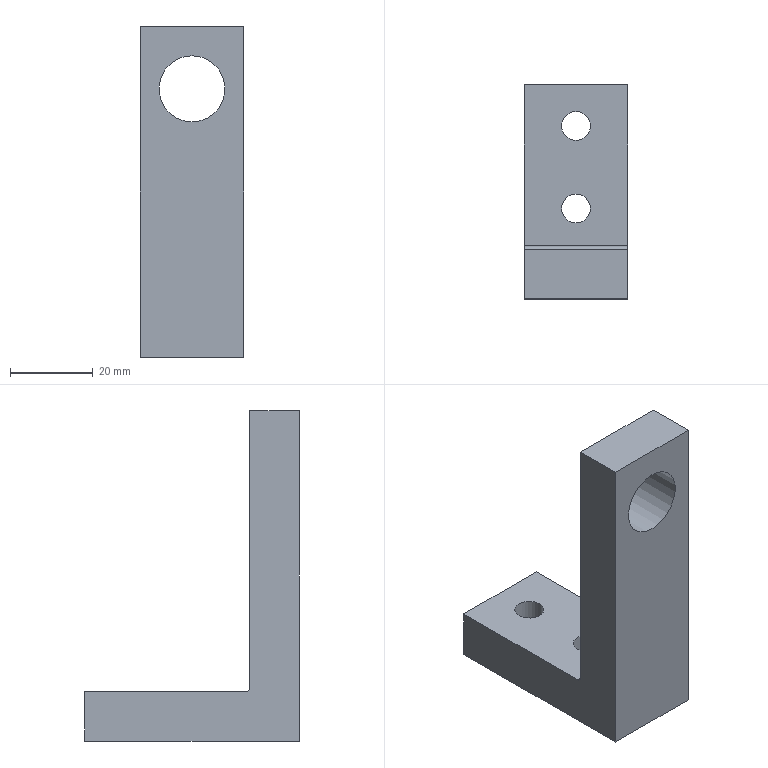Part | NX | features 5003_218_Panel feed stopper 2 | 1 solid | 12 faces | box 25 x 52 x 80 mm | volume 32669 mm3 | plane 8 | cylinder 4 | commonest cylinder face diameters 7 x2 2 x1 16 x1
STEP:
#1=CARTESIAN_POINT('',(-152.975,25.9,-107.));
#2=VERTEX_POINT('',#1);
#3=CARTESIAN_POINT('',(-152.975,13.9,-107.));
#4=VERTEX_POINT('',#3);
#5=CARTESIAN_POINT('',(-152.975,25.9,-107.));
#6=DIRECTION('',(0.,-1.,0.));
#7=VECTOR('',#6,1000.);
#8=LINE('',#5,#7);
#9=EDGE_CURVE('',#2,#4,#8,.T.);
#10=ORIENTED_EDGE('',*,*,#9,.T.);
#11=CARTESIAN_POINT('',(-127.975,13.9,-107.));
#12=VERTEX_POINT('',#11);
#13=CARTESIAN_POINT('',(-127.975,13.9,-107.));
#14=DIRECTION('',(-1.,0.,0.));
#15=VECTOR('',#14,1000.);
#16=LINE('',#13,#15);
#17=EDGE_CURVE('',#12,#4,#16,.T.);
#18=ORIENTED_EDGE('',*,*,#17,.F.);
#19=CARTESIAN_POINT('',(-127.975,25.9,-107.));
#20=VERTEX_POINT('',#19);
#21=CARTESIAN_POINT('',(-127.975,25.9,-107.));
#22=DIRECTION('',(0.,-1.,0.));
#23=VECTOR('',#22,1000.);
#24=LINE('',#21,#23);
#25=EDGE_CURVE('',#20,#12,#24,.T.);
#26=ORIENTED_EDGE('',*,*,#25,.F.);
#27=CARTESIAN_POINT('',(-127.975,25.9,-107.));
#28=DIRECTION('',(-1.,0.,0.));
#29=VECTOR('',#28,1000.);
#30=LINE('',#27,#29);
#31=EDGE_CURVE('',#20,#2,#30,.T.);
#32=ORIENTED_EDGE('',*,*,#31,.T.);
#33=EDGE_LOOP('',(#10,#18,#26,#32));
#34=FACE_BOUND('',#33,.T.);
#35=CARTESIAN_POINT('',(-127.975,25.9,-107.));
#36=DIRECTION('',(0.,0.,-1.));
#37=DIRECTION('',(0.,1.,0.));
#38=AXIS2_PLACEMENT_3D('',#35,#36,#37);
#39=PLANE('',#38);
#40=ADVANCED_FACE('',(#34),#39,.F.);
#41=CARTESIAN_POINT('',(-140.475,13.9,-114.));
#42=VERTEX_POINT('',#41);
#43=CARTESIAN_POINT('',(-140.475,13.9,-122.));
#44=DIRECTION('',(0.,1.,0.));
#45=DIRECTION('',(0.,0.,1.));
#46=AXIS2_PLACEMENT_3D('',#43,#44,#45);
#47=CIRCLE('',#46,8.);
#48=EDGE_CURVE('',#42,#42,#47,.T.);
#49=ORIENTED_EDGE('',*,*,#48,.T.);
#50=EDGE_LOOP('',(#49));
#51=FACE_BOUND('',#50,.T.);
#52=CARTESIAN_POINT('',(-152.975,13.9,-187.));
#53=VERTEX_POINT('',#52);
#54=CARTESIAN_POINT('',(-152.975,13.9,-107.));
#55=DIRECTION('',(0.,0.,-1.));
#56=VECTOR('',#55,1000.);
#57=LINE('',#54,#56);
#58=EDGE_CURVE('',#4,#53,#57,.T.);
#59=ORIENTED_EDGE('',*,*,#58,.T.);
#60=CARTESIAN_POINT('',(-127.975,13.9,-187.));
#61=VERTEX_POINT('',#60);
#62=CARTESIAN_POINT('',(-127.975,13.9,-187.));
#63=DIRECTION('',(-1.,0.,0.));
#64=VECTOR('',#63,1000.);
#65=LINE('',#62,#64);
#66=EDGE_CURVE('',#61,#53,#65,.T.);
#67=ORIENTED_EDGE('',*,*,#66,.F.);
#68=CARTESIAN_POINT('',(-127.975,13.9,-107.));
#69=DIRECTION('',(0.,0.,-1.));
#70=VECTOR('',#69,1000.);
#71=LINE('',#68,#70);
#72=EDGE_CURVE('',#12,#61,#71,.T.);
#73=ORIENTED_EDGE('',*,*,#72,.F.);
#74=ORIENTED_EDGE('',*,*,#17,.T.);
#75=EDGE_LOOP('',(#59,#67,#73,#74));
#76=FACE_BOUND('',#75,.T.);
#77=CARTESIAN_POINT('',(-127.975,13.9,-107.));
#78=DIRECTION('',(0.,1.,0.));
#79=DIRECTION('',(0.,0.,1.));
#80=AXIS2_PLACEMENT_3D('',#77,#78,#79);
#81=PLANE('',#80);
#82=ADVANCED_FACE('',(#51,#76),#81,.F.);
#83=CARTESIAN_POINT('',(-140.475,52.4,-187.));
#84=VERTEX_POINT('',#83);
#85=CARTESIAN_POINT('',(-140.475,55.9,-187.));
#86=DIRECTION('',(0.,0.,1.));
#87=DIRECTION('',(0.,-1.,0.));
#88=AXIS2_PLACEMENT_3D('',#85,#86,#87);
#89=CIRCLE('',#88,3.5);
#90=EDGE_CURVE('',#84,#84,#89,.T.);
#91=ORIENTED_EDGE('',*,*,#90,.T.);
#92=EDGE_LOOP('',(#91));
#93=FACE_BOUND('',#92,.T.);
#94=CARTESIAN_POINT('',(-140.475,32.4,-187.));
#95=VERTEX_POINT('',#94);
#96=CARTESIAN_POINT('',(-140.475,35.9,-187.));
#97=DIRECTION('',(0.,0.,1.));
#98=DIRECTION('',(0.,-1.,0.));
#99=AXIS2_PLACEMENT_3D('',#96,#97,#98);
#100=CIRCLE('',#99,3.5);
#101=EDGE_CURVE('',#95,#95,#100,.T.);
#102=ORIENTED_EDGE('',*,*,#101,.T.);
#103=EDGE_LOOP('',(#102));
#104=FACE_BOUND('',#103,.T.);
#105=CARTESIAN_POINT('',(-152.975,65.9,-187.));
#106=VERTEX_POINT('',#105);
#107=CARTESIAN_POINT('',(-152.975,13.9,-187.));
#108=DIRECTION('',(0.,1.,0.));
#109=VECTOR('',#108,1000.);
#110=LINE('',#107,#109);
#111=EDGE_CURVE('',#53,#106,#110,.T.);
#112=ORIENTED_EDGE('',*,*,#111,.T.);
#113=CARTESIAN_POINT('',(-127.975,65.9,-187.));
#114=VERTEX_POINT('',#113);
#115=CARTESIAN_POINT('',(-127.975,65.9,-187.));
#116=DIRECTION('',(-1.,0.,0.));
#117=VECTOR('',#116,1000.);
#118=LINE('',#115,#117);
#119=EDGE_CURVE('',#114,#106,#118,.T.);
#120=ORIENTED_EDGE('',*,*,#119,.F.);
#121=CARTESIAN_POINT('',(-127.975,13.9,-187.));
#122=DIRECTION('',(0.,1.,0.));
#123=VECTOR('',#122,1000.);
#124=LINE('',#121,#123);
#125=EDGE_CURVE('',#61,#114,#124,.T.);
#126=ORIENTED_EDGE('',*,*,#125,.F.);
#127=ORIENTED_EDGE('',*,*,#66,.T.);
#128=EDGE_LOOP('',(#112,#120,#126,#127));
#129=FACE_BOUND('',#128,.T.);
#130=CARTESIAN_POINT('',(-127.975,13.9,-187.));
#131=DIRECTION('',(0.,0.,1.));
#132=DIRECTION('',(0.,-1.,0.));
#133=AXIS2_PLACEMENT_3D('',#130,#131,#132);
#134=PLANE('',#133);
#135=ADVANCED_FACE('',(#93,#104,#129),#134,.F.);
#136=CARTESIAN_POINT('',(-152.975,65.9,-175.));
#137=VERTEX_POINT('',#136);
#138=CARTESIAN_POINT('',(-152.975,65.9,-187.));
#139=DIRECTION('',(0.,0.,1.));
#140=VECTOR('',#139,1000.);
#141=LINE('',#138,#140);
#142=EDGE_CURVE('',#106,#137,#141,.T.);
#143=ORIENTED_EDGE('',*,*,#142,.T.);
#144=CARTESIAN_POINT('',(-127.975,65.9,-175.));
#145=VERTEX_POINT('',#144);
#146=CARTESIAN_POINT('',(-127.975,65.9,-175.));
#147=DIRECTION('',(-1.,0.,0.));
#148=VECTOR('',#147,1000.);
#149=LINE('',#146,#148);
#150=EDGE_CURVE('',#145,#137,#149,.T.);
#151=ORIENTED_EDGE('',*,*,#150,.F.);
#152=CARTESIAN_POINT('',(-127.975,65.9,-187.));
#153=DIRECTION('',(0.,0.,1.));
#154=VECTOR('',#153,1000.);
#155=LINE('',#152,#154);
#156=EDGE_CURVE('',#114,#145,#155,.T.);
#157=ORIENTED_EDGE('',*,*,#156,.F.);
#158=ORIENTED_EDGE('',*,*,#119,.T.);
#159=EDGE_LOOP('',(#143,#151,#157,#158));
#160=FACE_BOUND('',#159,.T.);
#161=CARTESIAN_POINT('',(-127.975,65.9,-187.));
#162=DIRECTION('',(0.,-1.,0.));
#163=DIRECTION('',(1.,0.,0.));
#164=AXIS2_PLACEMENT_3D('',#161,#162,#163);
#165=PLANE('',#164);
#166=ADVANCED_FACE('',(#160),#165,.F.);
#167=CARTESIAN_POINT('',(-140.475,52.4,-175.));
#168=VERTEX_POINT('',#167);
#169=CARTESIAN_POINT('',(-140.475,55.9,-175.));
#170=DIRECTION('',(0.,0.,1.));
#171=DIRECTION('',(0.,-1.,0.));
#172=AXIS2_PLACEMENT_3D('',#169,#170,#171);
#173=CIRCLE('',#172,3.5);
#174=EDGE_CURVE('',#168,#168,#173,.T.);
#175=ORIENTED_EDGE('',*,*,#174,.F.);
#176=EDGE_LOOP('',(#175));
#177=FACE_BOUND('',#176,.T.);
#178=CARTESIAN_POINT('',(-140.475,32.4,-175.));
#179=VERTEX_POINT('',#178);
#180=CARTESIAN_POINT('',(-140.475,35.9,-175.));
#181=DIRECTION('',(0.,0.,1.));
#182=DIRECTION('',(0.,-1.,0.));
#183=AXIS2_PLACEMENT_3D('',#180,#181,#182);
#184=CIRCLE('',#183,3.5);
#185=EDGE_CURVE('',#179,#179,#184,.T.);
#186=ORIENTED_EDGE('',*,*,#185,.F.);
#187=EDGE_LOOP('',(#186));
#188=FACE_BOUND('',#187,.T.);
#189=CARTESIAN_POINT('',(-152.975,26.9,-175.));
#190=VERTEX_POINT('',#189);
#191=CARTESIAN_POINT('',(-152.975,65.9,-175.));
#192=DIRECTION('',(0.,-1.,0.));
#193=VECTOR('',#192,1000.);
#194=LINE('',#191,#193);
#195=EDGE_CURVE('',#137,#190,#194,.T.);
#196=ORIENTED_EDGE('',*,*,#195,.T.);
#197=CARTESIAN_POINT('',(-127.975,26.9,-175.));
#198=VERTEX_POINT('',#197);
#199=CARTESIAN_POINT('',(-127.975,26.9,-175.));
#200=DIRECTION('',(-1.,0.,0.));
#201=VECTOR('',#200,1000.);
#202=LINE('',#199,#201);
#203=EDGE_CURVE('',#190,#198,#202,.F.);
#204=ORIENTED_EDGE('',*,*,#203,.T.);
#205=CARTESIAN_POINT('',(-127.975,65.9,-175.));
#206=DIRECTION('',(0.,-1.,0.));
#207=VECTOR('',#206,1000.);
#208=LINE('',#205,#207);
#209=EDGE_CURVE('',#145,#198,#208,.T.);
#210=ORIENTED_EDGE('',*,*,#209,.F.);
#211=ORIENTED_EDGE('',*,*,#150,.T.);
#212=EDGE_LOOP('',(#196,#204,#210,#211));
#213=FACE_BOUND('',#212,.T.);
#214=CARTESIAN_POINT('',(-127.975,65.9,-175.));
#215=DIRECTION('',(0.,0.,-1.));
#216=DIRECTION('',(0.,1.,0.));
#217=AXIS2_PLACEMENT_3D('',#214,#215,#216);
#218=PLANE('',#217);
#219=ADVANCED_FACE('',(#177,#188,#213),#218,.F.);
#220=CARTESIAN_POINT('',(-140.475,25.9,-114.));
#221=VERTEX_POINT('',#220);
#222=CARTESIAN_POINT('',(-140.475,25.9,-122.));
#223=DIRECTION('',(0.,1.,0.));
#224=DIRECTION('',(0.,0.,1.));
#225=AXIS2_PLACEMENT_3D('',#222,#223,#224);
#226=CIRCLE('',#225,8.);
#227=EDGE_CURVE('',#221,#221,#226,.T.);
#228=ORIENTED_EDGE('',*,*,#227,.F.);
#229=EDGE_LOOP('',(#228));
#230=FACE_BOUND('',#229,.T.);
#231=CARTESIAN_POINT('',(-127.975,25.9,-174.));
#232=VERTEX_POINT('',#231);
#233=CARTESIAN_POINT('',(-127.975,25.9,-175.));
#234=DIRECTION('',(0.,0.,1.));
#235=VECTOR('',#234,1000.);
#236=LINE('',#233,#235);
#237=EDGE_CURVE('',#232,#20,#236,.T.);
#238=ORIENTED_EDGE('',*,*,#237,.F.);
#239=CARTESIAN_POINT('',(-152.975,25.9,-174.));
#240=VERTEX_POINT('',#239);
#241=CARTESIAN_POINT('',(-152.975,25.9,-174.));
#242=DIRECTION('',(-1.,0.,0.));
#243=VECTOR('',#242,1000.);
#244=LINE('',#241,#243);
#245=EDGE_CURVE('',#232,#240,#244,.T.);
#246=ORIENTED_EDGE('',*,*,#245,.T.);
#247=CARTESIAN_POINT('',(-152.975,25.9,-175.));
#248=DIRECTION('',(0.,0.,1.));
#249=VECTOR('',#248,1000.);
#250=LINE('',#247,#249);
#251=EDGE_CURVE('',#240,#2,#250,.T.);
#252=ORIENTED_EDGE('',*,*,#251,.T.);
#253=ORIENTED_EDGE('',*,*,#31,.F.);
#254=EDGE_LOOP('',(#238,#246,#252,#253));
#255=FACE_BOUND('',#254,.T.);
#256=CARTESIAN_POINT('',(-127.975,25.9,-175.));
#257=DIRECTION('',(0.,-1.,0.));
#258=DIRECTION('',(0.,0.,-1.));
#259=AXIS2_PLACEMENT_3D('',#256,#257,#258);
#260=PLANE('',#259);
#261=ADVANCED_FACE('',(#230,#255),#260,.F.);
#262=ORIENTED_EDGE('',*,*,#25,.T.);
#263=ORIENTED_EDGE('',*,*,#72,.T.);
#264=ORIENTED_EDGE('',*,*,#125,.T.);
#265=ORIENTED_EDGE('',*,*,#156,.T.);
#266=ORIENTED_EDGE('',*,*,#209,.T.);
#267=CARTESIAN_POINT('',(-127.975,26.9,-174.));
#268=DIRECTION('',(1.,0.,0.));
#269=DIRECTION('',(0.,1.,0.));
#270=AXIS2_PLACEMENT_3D('',#267,#268,#269);
#271=CIRCLE('',#270,1.);
#272=EDGE_CURVE('',#198,#232,#271,.F.);
#273=ORIENTED_EDGE('',*,*,#272,.T.);
#274=ORIENTED_EDGE('',*,*,#237,.T.);
#275=EDGE_LOOP('',(#262,#263,#264,#265,#266,#273,#274));
#276=FACE_BOUND('',#275,.T.);
#277=CARTESIAN_POINT('',(-127.975,13.9,-187.));
#278=DIRECTION('',(1.,0.,0.));
#279=DIRECTION('',(0.,1.,0.));
#280=AXIS2_PLACEMENT_3D('',#277,#278,#279);
#281=PLANE('',#280);
#282=ADVANCED_FACE('',(#276),#281,.T.);
#283=ORIENTED_EDGE('',*,*,#9,.F.);
#284=ORIENTED_EDGE('',*,*,#251,.F.);
#285=CARTESIAN_POINT('',(-152.975,26.9,-174.));
#286=DIRECTION('',(1.,0.,0.));
#287=DIRECTION('',(0.,1.,0.));
#288=AXIS2_PLACEMENT_3D('',#285,#286,#287);
#289=CIRCLE('',#288,1.);
#290=EDGE_CURVE('',#240,#190,#289,.T.);
#291=ORIENTED_EDGE('',*,*,#290,.T.);
#292=ORIENTED_EDGE('',*,*,#195,.F.);
#293=ORIENTED_EDGE('',*,*,#142,.F.);
#294=ORIENTED_EDGE('',*,*,#111,.F.);
#295=ORIENTED_EDGE('',*,*,#58,.F.);
#296=EDGE_LOOP('',(#283,#284,#291,#292,#293,#294,#295));
#297=FACE_BOUND('',#296,.T.);
#298=CARTESIAN_POINT('',(-152.975,13.9,-187.));
#299=DIRECTION('',(1.,0.,0.));
#300=DIRECTION('',(0.,1.,0.));
#301=AXIS2_PLACEMENT_3D('',#298,#299,#300);
#302=PLANE('',#301);
#303=ADVANCED_FACE('',(#297),#302,.F.);
#304=ORIENTED_EDGE('',*,*,#48,.F.);
#305=EDGE_LOOP('',(#304));
#306=FACE_BOUND('',#305,.T.);
#307=ORIENTED_EDGE('',*,*,#227,.T.);
#308=EDGE_LOOP('',(#307));
#309=FACE_BOUND('',#308,.T.);
#310=CARTESIAN_POINT('',(-140.475,25.9,-122.));
#311=DIRECTION('',(0.,1.,0.));
#312=DIRECTION('',(0.,0.,1.));
#313=AXIS2_PLACEMENT_3D('',#310,#311,#312);
#314=CYLINDRICAL_SURFACE('',#313,8.);
#315=ADVANCED_FACE('',(#306,#309),#314,.F.);
#316=ORIENTED_EDGE('',*,*,#101,.F.);
#317=EDGE_LOOP('',(#316));
#318=FACE_BOUND('',#317,.T.);
#319=ORIENTED_EDGE('',*,*,#185,.T.);
#320=EDGE_LOOP('',(#319));
#321=FACE_BOUND('',#320,.T.);
#322=CARTESIAN_POINT('',(-140.475,35.9,-175.));
#323=DIRECTION('',(0.,0.,1.));
#324=DIRECTION('',(0.,-1.,0.));
#325=AXIS2_PLACEMENT_3D('',#322,#323,#324);
#326=CYLINDRICAL_SURFACE('',#325,3.5);
#327=ADVANCED_FACE('',(#318,#321),#326,.F.);
#328=ORIENTED_EDGE('',*,*,#90,.F.);
#329=EDGE_LOOP('',(#328));
#330=FACE_BOUND('',#329,.T.);
#331=ORIENTED_EDGE('',*,*,#174,.T.);
#332=EDGE_LOOP('',(#331));
#333=FACE_BOUND('',#332,.T.);
#334=CARTESIAN_POINT('',(-140.475,55.9,-175.));
#335=DIRECTION('',(0.,0.,1.));
#336=DIRECTION('',(0.,-1.,0.));
#337=AXIS2_PLACEMENT_3D('',#334,#335,#336);
#338=CYLINDRICAL_SURFACE('',#337,3.5);
#339=ADVANCED_FACE('',(#330,#333),#338,.F.);
#340=ORIENTED_EDGE('',*,*,#272,.F.);
#341=ORIENTED_EDGE('',*,*,#203,.F.);
#342=ORIENTED_EDGE('',*,*,#290,.F.);
#343=ORIENTED_EDGE('',*,*,#245,.F.);
#344=EDGE_LOOP('',(#340,#341,#342,#343));
#345=FACE_BOUND('',#344,.T.);
#346=CARTESIAN_POINT('',(-127.975,26.9,-174.));
#347=DIRECTION('',(1.,0.,0.));
#348=DIRECTION('',(0.,1.,0.));
#349=AXIS2_PLACEMENT_3D('',#346,#347,#348);
#350=CYLINDRICAL_SURFACE('',#349,1.);
#351=ADVANCED_FACE('',(#345),#350,.F.);
#352=CLOSED_SHELL('',(#40,#82,#135,#166,#219,#261,#282,#303,#315,#327,#339,#351));
#353=MANIFOLD_SOLID_BREP('',#352);
#354=(LENGTH_UNIT()NAMED_UNIT(*)SI_UNIT(.MILLI.,.METRE.));
#355=UNCERTAINTY_MEASURE_WITH_UNIT(LENGTH_MEASURE(0.00001),#354,'','');
#356=(NAMED_UNIT(*)PLANE_ANGLE_UNIT()SI_UNIT($,.RADIAN.));
#357=(NAMED_UNIT(*)SI_UNIT($,.STERADIAN.)SOLID_ANGLE_UNIT());
#358=(GEOMETRIC_REPRESENTATION_CONTEXT(3)GLOBAL_UNCERTAINTY_ASSIGNED_CONTEXT((#355))GLOBAL_UNIT_ASSIGNED_CONTEXT((#354,#356,#357))REPRESENTATION_CONTEXT('',''));
#359=ADVANCED_BREP_SHAPE_REPRESENTATION('',(#353),#358);